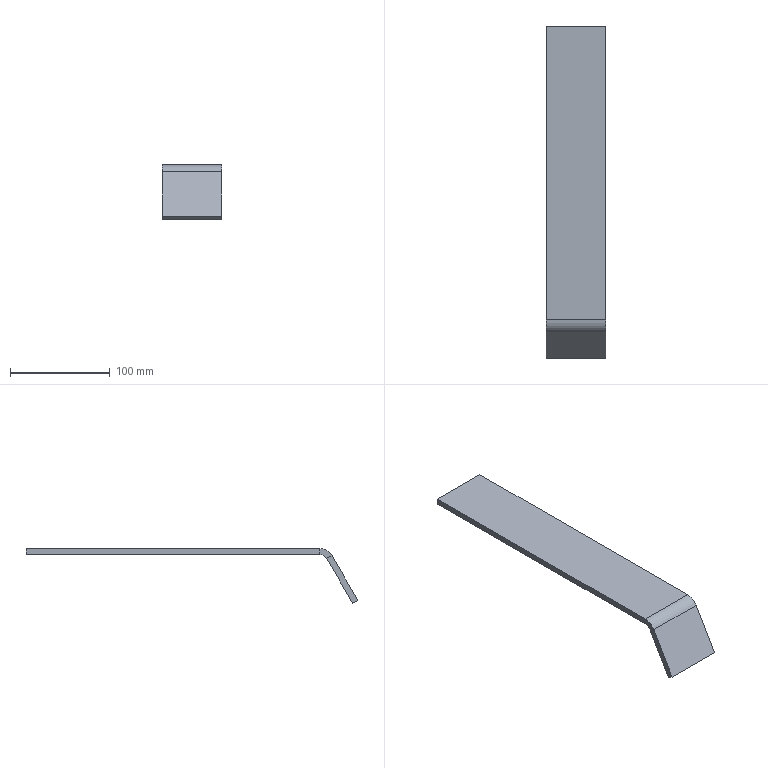Part | SolidWorks | features FlatPattern 1, SMBaseFlange 1, SheetMetal 1 | 1 solid | 14 faces | box 60 x 332 x 54.962 mm | volume 128647 mm3 | plane 12 | cylinder 2 | commonest cylinder face diameters 16 x1 28 x1
STEP:
#1=CARTESIAN_POINT('',(60.,8.083,0.));
#2=VERTEX_POINT('',#1);
#3=CARTESIAN_POINT('',(60.,8.083,-6.));
#4=VERTEX_POINT('',#3);
#5=CARTESIAN_POINT('',(60.,8.083,0.));
#6=DIRECTION('',(0.,0.,-1.));
#7=VECTOR('',#6,1000.);
#8=LINE('',#5,#7);
#9=EDGE_CURVE('',#2,#4,#8,.T.);
#10=ORIENTED_EDGE('',*,*,#9,.F.);
#11=CARTESIAN_POINT('',(60.,-4.041,-7.));
#12=VERTEX_POINT('',#11);
#13=CARTESIAN_POINT('',(60.,8.083,-14.));
#14=DIRECTION('',(1.,0.,0.));
#15=DIRECTION('',(0.,0.,1.));
#16=AXIS2_PLACEMENT_3D('',#13,#14,#15);
#17=CIRCLE('',#16,14.);
#18=EDGE_CURVE('',#2,#12,#17,.T.);
#19=ORIENTED_EDGE('',*,*,#18,.T.);
#20=CARTESIAN_POINT('',(60.,1.155,-10.));
#21=VERTEX_POINT('',#20);
#22=CARTESIAN_POINT('',(60.,1.155,-10.));
#23=DIRECTION('',(0.,-0.866,0.5));
#24=VECTOR('',#23,1000.);
#25=LINE('',#22,#24);
#26=EDGE_CURVE('',#21,#12,#25,.T.);
#27=ORIENTED_EDGE('',*,*,#26,.F.);
#28=CARTESIAN_POINT('',(60.,8.083,-14.));
#29=DIRECTION('',(1.,0.,0.));
#30=DIRECTION('',(0.,0.,-1.));
#31=AXIS2_PLACEMENT_3D('',#28,#29,#30);
#32=CIRCLE('',#31,8.);
#33=EDGE_CURVE('',#4,#21,#32,.T.);
#34=ORIENTED_EDGE('',*,*,#33,.F.);
#35=EDGE_LOOP('',(#10,#19,#27,#34));
#36=FACE_OUTER_BOUND('',#35,.T.);
#37=CARTESIAN_POINT('',(60.,8.083,0.));
#38=DIRECTION('',(1.,0.,0.));
#39=DIRECTION('',(0.,0.,-1.));
#40=AXIS2_PLACEMENT_3D('',#37,#38,#39);
#41=PLANE('',#40);
#42=ADVANCED_FACE('',(#36),#41,.T.);
#43=CARTESIAN_POINT('',(60.,302.,0.));
#44=VERTEX_POINT('',#43);
#45=CARTESIAN_POINT('',(60.,0.,0.));
#46=DIRECTION('',(0.,-1.,0.));
#47=VECTOR('',#46,1000.);
#48=LINE('',#45,#47);
#49=EDGE_CURVE('',#44,#2,#48,.T.);
#50=ORIENTED_EDGE('',*,*,#49,.T.);
#51=ORIENTED_EDGE('',*,*,#9,.T.);
#52=CARTESIAN_POINT('',(60.,302.,-6.));
#53=VERTEX_POINT('',#52);
#54=CARTESIAN_POINT('',(60.,0.,-6.));
#55=DIRECTION('',(0.,-1.,0.));
#56=VECTOR('',#55,1000.);
#57=LINE('',#54,#56);
#58=EDGE_CURVE('',#53,#4,#57,.T.);
#59=ORIENTED_EDGE('',*,*,#58,.F.);
#60=CARTESIAN_POINT('',(60.,302.,0.));
#61=DIRECTION('',(0.,0.,-1.));
#62=VECTOR('',#61,1000.);
#63=LINE('',#60,#62);
#64=EDGE_CURVE('',#44,#53,#63,.T.);
#65=ORIENTED_EDGE('',*,*,#64,.F.);
#66=EDGE_LOOP('',(#50,#51,#59,#65));
#67=FACE_OUTER_BOUND('',#66,.T.);
#68=CARTESIAN_POINT('',(60.,1.155,-10.));
#69=DIRECTION('',(1.,0.,0.));
#70=DIRECTION('',(0.,0.,-1.));
#71=AXIS2_PLACEMENT_3D('',#68,#69,#70);
#72=PLANE('',#71);
#73=ADVANCED_FACE('',(#67),#72,.T.);
#74=CARTESIAN_POINT('',(0.,-4.041,-7.));
#75=VERTEX_POINT('',#74);
#76=CARTESIAN_POINT('',(0.,1.155,-10.));
#77=VERTEX_POINT('',#76);
#78=CARTESIAN_POINT('',(0.,-4.041,-7.));
#79=DIRECTION('',(0.,0.866,-0.5));
#80=VECTOR('',#79,1000.);
#81=LINE('',#78,#80);
#82=EDGE_CURVE('',#75,#77,#81,.T.);
#83=ORIENTED_EDGE('',*,*,#82,.F.);
#84=CARTESIAN_POINT('',(0.,8.083,0.));
#85=VERTEX_POINT('',#84);
#86=CARTESIAN_POINT('',(0.,8.083,-14.));
#87=DIRECTION('',(1.,0.,0.));
#88=DIRECTION('',(0.,0.,1.));
#89=AXIS2_PLACEMENT_3D('',#86,#87,#88);
#90=CIRCLE('',#89,14.);
#91=EDGE_CURVE('',#85,#75,#90,.T.);
#92=ORIENTED_EDGE('',*,*,#91,.F.);
#93=CARTESIAN_POINT('',(0.,8.083,-6.));
#94=VERTEX_POINT('',#93);
#95=CARTESIAN_POINT('',(0.,8.083,-6.));
#96=DIRECTION('',(0.,0.,1.));
#97=VECTOR('',#96,1000.);
#98=LINE('',#95,#97);
#99=EDGE_CURVE('',#94,#85,#98,.T.);
#100=ORIENTED_EDGE('',*,*,#99,.F.);
#101=CARTESIAN_POINT('',(0.,8.083,-14.));
#102=DIRECTION('',(1.,0.,0.));
#103=DIRECTION('',(0.,0.,-1.));
#104=AXIS2_PLACEMENT_3D('',#101,#102,#103);
#105=CIRCLE('',#104,8.);
#106=EDGE_CURVE('',#94,#77,#105,.T.);
#107=ORIENTED_EDGE('',*,*,#106,.T.);
#108=EDGE_LOOP('',(#83,#92,#100,#107));
#109=FACE_OUTER_BOUND('',#108,.T.);
#110=CARTESIAN_POINT('',(0.,-4.041,-7.));
#111=DIRECTION('',(-1.,0.,0.));
#112=DIRECTION('',(0.,0.,1.));
#113=AXIS2_PLACEMENT_3D('',#110,#111,#112);
#114=PLANE('',#113);
#115=ADVANCED_FACE('',(#109),#114,.T.);
#116=CARTESIAN_POINT('',(0.,-30.,-51.962));
#117=VERTEX_POINT('',#116);
#118=CARTESIAN_POINT('',(0.,0.,0.));
#119=DIRECTION('',(0.,-0.5,-0.866));
#120=VECTOR('',#119,1000.);
#121=LINE('',#118,#120);
#122=EDGE_CURVE('',#75,#117,#121,.T.);
#123=ORIENTED_EDGE('',*,*,#122,.F.);
#124=ORIENTED_EDGE('',*,*,#82,.T.);
#125=CARTESIAN_POINT('',(0.,-24.804,-54.962));
#126=VERTEX_POINT('',#125);
#127=CARTESIAN_POINT('',(0.,5.196,-3.));
#128=DIRECTION('',(0.,-0.5,-0.866));
#129=VECTOR('',#128,1000.);
#130=LINE('',#127,#129);
#131=EDGE_CURVE('',#77,#126,#130,.T.);
#132=ORIENTED_EDGE('',*,*,#131,.T.);
#133=CARTESIAN_POINT('',(0.,-24.804,-54.962));
#134=DIRECTION('',(0.,-0.866,0.5));
#135=VECTOR('',#134,1000.);
#136=LINE('',#133,#135);
#137=EDGE_CURVE('',#126,#117,#136,.T.);
#138=ORIENTED_EDGE('',*,*,#137,.T.);
#139=EDGE_LOOP('',(#123,#124,#132,#138));
#140=FACE_OUTER_BOUND('',#139,.T.);
#141=CARTESIAN_POINT('',(0.,8.083,-6.));
#142=DIRECTION('',(-1.,0.,0.));
#143=DIRECTION('',(0.,0.,1.));
#144=AXIS2_PLACEMENT_3D('',#141,#142,#143);
#145=PLANE('',#144);
#146=ADVANCED_FACE('',(#140),#145,.T.);
#147=ORIENTED_EDGE('',*,*,#122,.T.);
#148=CARTESIAN_POINT('',(60.,-30.,-51.962));
#149=VERTEX_POINT('',#148);
#150=CARTESIAN_POINT('',(60.,-30.,-51.962));
#151=DIRECTION('',(-1.,0.,0.));
#152=VECTOR('',#151,1000.);
#153=LINE('',#150,#152);
#154=EDGE_CURVE('',#149,#117,#153,.T.);
#155=ORIENTED_EDGE('',*,*,#154,.F.);
#156=CARTESIAN_POINT('',(60.,0.,0.));
#157=DIRECTION('',(0.,-0.5,-0.866));
#158=VECTOR('',#157,1000.);
#159=LINE('',#156,#158);
#160=EDGE_CURVE('',#12,#149,#159,.T.);
#161=ORIENTED_EDGE('',*,*,#160,.F.);
#162=CARTESIAN_POINT('',(60.,-4.041,-7.));
#163=DIRECTION('',(-1.,0.,0.));
#164=VECTOR('',#163,1000.);
#165=LINE('',#162,#164);
#166=EDGE_CURVE('',#12,#75,#165,.T.);
#167=ORIENTED_EDGE('',*,*,#166,.T.);
#168=EDGE_LOOP('',(#147,#155,#161,#167));
#169=FACE_OUTER_BOUND('',#168,.T.);
#170=CARTESIAN_POINT('',(60.,0.,0.));
#171=DIRECTION('',(0.,0.866,-0.5));
#172=DIRECTION('',(0.,0.5,0.866));
#173=AXIS2_PLACEMENT_3D('',#170,#171,#172);
#174=PLANE('',#173);
#175=ADVANCED_FACE('',(#169),#174,.F.);
#176=ORIENTED_EDGE('',*,*,#137,.F.);
#177=CARTESIAN_POINT('',(60.,-24.804,-54.962));
#178=VERTEX_POINT('',#177);
#179=CARTESIAN_POINT('',(60.,-24.804,-54.962));
#180=DIRECTION('',(-1.,0.,0.));
#181=VECTOR('',#180,1000.);
#182=LINE('',#179,#181);
#183=EDGE_CURVE('',#178,#126,#182,.T.);
#184=ORIENTED_EDGE('',*,*,#183,.F.);
#185=CARTESIAN_POINT('',(60.,-24.804,-54.962));
#186=DIRECTION('',(0.,-0.866,0.5));
#187=VECTOR('',#186,1000.);
#188=LINE('',#185,#187);
#189=EDGE_CURVE('',#178,#149,#188,.T.);
#190=ORIENTED_EDGE('',*,*,#189,.T.);
#191=ORIENTED_EDGE('',*,*,#154,.T.);
#192=EDGE_LOOP('',(#176,#184,#190,#191));
#193=FACE_OUTER_BOUND('',#192,.T.);
#194=CARTESIAN_POINT('',(60.,-24.804,-54.962));
#195=DIRECTION('',(0.,-0.5,-0.866));
#196=DIRECTION('',(0.,0.866,-0.5));
#197=AXIS2_PLACEMENT_3D('',#194,#195,#196);
#198=PLANE('',#197);
#199=ADVANCED_FACE('',(#193),#198,.T.);
#200=ORIENTED_EDGE('',*,*,#131,.F.);
#201=CARTESIAN_POINT('',(60.,1.155,-10.));
#202=DIRECTION('',(-1.,0.,0.));
#203=VECTOR('',#202,1000.);
#204=LINE('',#201,#203);
#205=EDGE_CURVE('',#21,#77,#204,.T.);
#206=ORIENTED_EDGE('',*,*,#205,.F.);
#207=CARTESIAN_POINT('',(60.,5.196,-3.));
#208=DIRECTION('',(0.,-0.5,-0.866));
#209=VECTOR('',#208,1000.);
#210=LINE('',#207,#209);
#211=EDGE_CURVE('',#21,#178,#210,.T.);
#212=ORIENTED_EDGE('',*,*,#211,.T.);
#213=ORIENTED_EDGE('',*,*,#183,.T.);
#214=EDGE_LOOP('',(#200,#206,#212,#213));
#215=FACE_OUTER_BOUND('',#214,.T.);
#216=CARTESIAN_POINT('',(60.,5.196,-3.));
#217=DIRECTION('',(0.,0.866,-0.5));
#218=DIRECTION('',(0.,0.5,0.866));
#219=AXIS2_PLACEMENT_3D('',#216,#217,#218);
#220=PLANE('',#219);
#221=ADVANCED_FACE('',(#215),#220,.T.);
#222=ORIENTED_EDGE('',*,*,#106,.F.);
#223=CARTESIAN_POINT('',(60.,8.083,-6.));
#224=DIRECTION('',(-1.,0.,0.));
#225=VECTOR('',#224,1000.);
#226=LINE('',#223,#225);
#227=EDGE_CURVE('',#4,#94,#226,.T.);
#228=ORIENTED_EDGE('',*,*,#227,.F.);
#229=ORIENTED_EDGE('',*,*,#33,.T.);
#230=ORIENTED_EDGE('',*,*,#205,.T.);
#231=EDGE_LOOP('',(#222,#228,#229,#230));
#232=FACE_OUTER_BOUND('',#231,.T.);
#233=CARTESIAN_POINT('',(60.,8.083,-14.));
#234=DIRECTION('',(-1.,0.,0.));
#235=DIRECTION('',(0.,0.,1.));
#236=AXIS2_PLACEMENT_3D('',#233,#234,#235);
#237=CYLINDRICAL_SURFACE('',#236,8.);
#238=ADVANCED_FACE('',(#232),#237,.F.);
#239=CARTESIAN_POINT('',(0.,302.,-6.));
#240=VERTEX_POINT('',#239);
#241=CARTESIAN_POINT('',(0.,0.,-6.));
#242=DIRECTION('',(0.,-1.,0.));
#243=VECTOR('',#242,1000.);
#244=LINE('',#241,#243);
#245=EDGE_CURVE('',#240,#94,#244,.T.);
#246=ORIENTED_EDGE('',*,*,#245,.F.);
#247=CARTESIAN_POINT('',(60.,302.,-6.));
#248=DIRECTION('',(-1.,0.,0.));
#249=VECTOR('',#248,1000.);
#250=LINE('',#247,#249);
#251=EDGE_CURVE('',#53,#240,#250,.T.);
#252=ORIENTED_EDGE('',*,*,#251,.F.);
#253=ORIENTED_EDGE('',*,*,#58,.T.);
#254=ORIENTED_EDGE('',*,*,#227,.T.);
#255=EDGE_LOOP('',(#246,#252,#253,#254));
#256=FACE_OUTER_BOUND('',#255,.T.);
#257=CARTESIAN_POINT('',(60.,0.,-6.));
#258=DIRECTION('',(0.,0.,-1.));
#259=DIRECTION('',(-1.,0.,0.));
#260=AXIS2_PLACEMENT_3D('',#257,#258,#259);
#261=PLANE('',#260);
#262=ADVANCED_FACE('',(#256),#261,.T.);
#263=CARTESIAN_POINT('',(0.,302.,0.));
#264=VERTEX_POINT('',#263);
#265=CARTESIAN_POINT('',(0.,302.,0.));
#266=DIRECTION('',(0.,0.,-1.));
#267=VECTOR('',#266,1000.);
#268=LINE('',#265,#267);
#269=EDGE_CURVE('',#264,#240,#268,.T.);
#270=ORIENTED_EDGE('',*,*,#269,.F.);
#271=CARTESIAN_POINT('',(60.,302.,0.));
#272=DIRECTION('',(-1.,0.,0.));
#273=VECTOR('',#272,1000.);
#274=LINE('',#271,#273);
#275=EDGE_CURVE('',#44,#264,#274,.T.);
#276=ORIENTED_EDGE('',*,*,#275,.F.);
#277=ORIENTED_EDGE('',*,*,#64,.T.);
#278=ORIENTED_EDGE('',*,*,#251,.T.);
#279=EDGE_LOOP('',(#270,#276,#277,#278));
#280=FACE_OUTER_BOUND('',#279,.T.);
#281=CARTESIAN_POINT('',(60.,302.,0.));
#282=DIRECTION('',(0.,1.,0.));
#283=DIRECTION('',(0.,0.,1.));
#284=AXIS2_PLACEMENT_3D('',#281,#282,#283);
#285=PLANE('',#284);
#286=ADVANCED_FACE('',(#280),#285,.T.);
#287=CARTESIAN_POINT('',(0.,0.,0.));
#288=DIRECTION('',(0.,-1.,0.));
#289=VECTOR('',#288,1000.);
#290=LINE('',#287,#289);
#291=EDGE_CURVE('',#264,#85,#290,.T.);
#292=ORIENTED_EDGE('',*,*,#291,.T.);
#293=CARTESIAN_POINT('',(60.,8.083,0.));
#294=DIRECTION('',(-1.,0.,0.));
#295=VECTOR('',#294,1000.);
#296=LINE('',#293,#295);
#297=EDGE_CURVE('',#2,#85,#296,.T.);
#298=ORIENTED_EDGE('',*,*,#297,.F.);
#299=ORIENTED_EDGE('',*,*,#49,.F.);
#300=ORIENTED_EDGE('',*,*,#275,.T.);
#301=EDGE_LOOP('',(#292,#298,#299,#300));
#302=FACE_OUTER_BOUND('',#301,.T.);
#303=CARTESIAN_POINT('',(60.,0.,0.));
#304=DIRECTION('',(0.,0.,-1.));
#305=DIRECTION('',(-1.,0.,0.));
#306=AXIS2_PLACEMENT_3D('',#303,#304,#305);
#307=PLANE('',#306);
#308=ADVANCED_FACE('',(#302),#307,.F.);
#309=ORIENTED_EDGE('',*,*,#91,.T.);
#310=ORIENTED_EDGE('',*,*,#166,.F.);
#311=ORIENTED_EDGE('',*,*,#18,.F.);
#312=ORIENTED_EDGE('',*,*,#297,.T.);
#313=EDGE_LOOP('',(#309,#310,#311,#312));
#314=FACE_OUTER_BOUND('',#313,.T.);
#315=CARTESIAN_POINT('',(60.,8.083,-14.));
#316=DIRECTION('',(-1.,0.,0.));
#317=DIRECTION('',(0.,0.,1.));
#318=AXIS2_PLACEMENT_3D('',#315,#316,#317);
#319=CYLINDRICAL_SURFACE('',#318,14.);
#320=ADVANCED_FACE('',(#314),#319,.T.);
#321=ORIENTED_EDGE('',*,*,#160,.T.);
#322=ORIENTED_EDGE('',*,*,#189,.F.);
#323=ORIENTED_EDGE('',*,*,#211,.F.);
#324=ORIENTED_EDGE('',*,*,#26,.T.);
#325=EDGE_LOOP('',(#321,#322,#323,#324));
#326=FACE_OUTER_BOUND('',#325,.T.);
#327=CARTESIAN_POINT('',(60.,8.083,-14.));
#328=DIRECTION('',(1.,0.,0.));
#329=DIRECTION('',(0.,0.,-1.));
#330=AXIS2_PLACEMENT_3D('',#327,#328,#329);
#331=PLANE('',#330);
#332=ADVANCED_FACE('',(#326),#331,.T.);
#333=ORIENTED_EDGE('',*,*,#245,.T.);
#334=ORIENTED_EDGE('',*,*,#99,.T.);
#335=ORIENTED_EDGE('',*,*,#291,.F.);
#336=ORIENTED_EDGE('',*,*,#269,.T.);
#337=EDGE_LOOP('',(#333,#334,#335,#336));
#338=FACE_OUTER_BOUND('',#337,.T.);
#339=CARTESIAN_POINT('',(0.,8.083,-14.));
#340=DIRECTION('',(1.,0.,0.));
#341=DIRECTION('',(0.,0.,-1.));
#342=AXIS2_PLACEMENT_3D('',#339,#340,#341);
#343=PLANE('',#342);
#344=ADVANCED_FACE('',(#338),#343,.F.);
#345=CLOSED_SHELL('',(#42,#73,#115,#146,#175,#199,#221,#238,#262,#286,#308,#320,#332,#344));
#346=MANIFOLD_SOLID_BREP('',#345);
#347=CARTESIAN_POINT('',(0.,0.,0.));
#348=DIRECTION('',(0.,0.,1.));
#349=DIRECTION('',(1.,0.,0.));
#350=AXIS2_PLACEMENT_3D('',#347,#348,#349);
#351=(LENGTH_UNIT()NAMED_UNIT(*)SI_UNIT(.MILLI.,.METRE.));
#352=UNCERTAINTY_MEASURE_WITH_UNIT(LENGTH_MEASURE(0.00001),#351,'','');
#353=(NAMED_UNIT(*)PLANE_ANGLE_UNIT()SI_UNIT($,.RADIAN.));
#354=(NAMED_UNIT(*)SI_UNIT($,.STERADIAN.)SOLID_ANGLE_UNIT());
#355=(GEOMETRIC_REPRESENTATION_CONTEXT(3)GLOBAL_UNCERTAINTY_ASSIGNED_CONTEXT((#352))GLOBAL_UNIT_ASSIGNED_CONTEXT((#351,#353,#354))REPRESENTATION_CONTEXT('',''));
#356=ADVANCED_BREP_SHAPE_REPRESENTATION('',(#346,#350),#355);